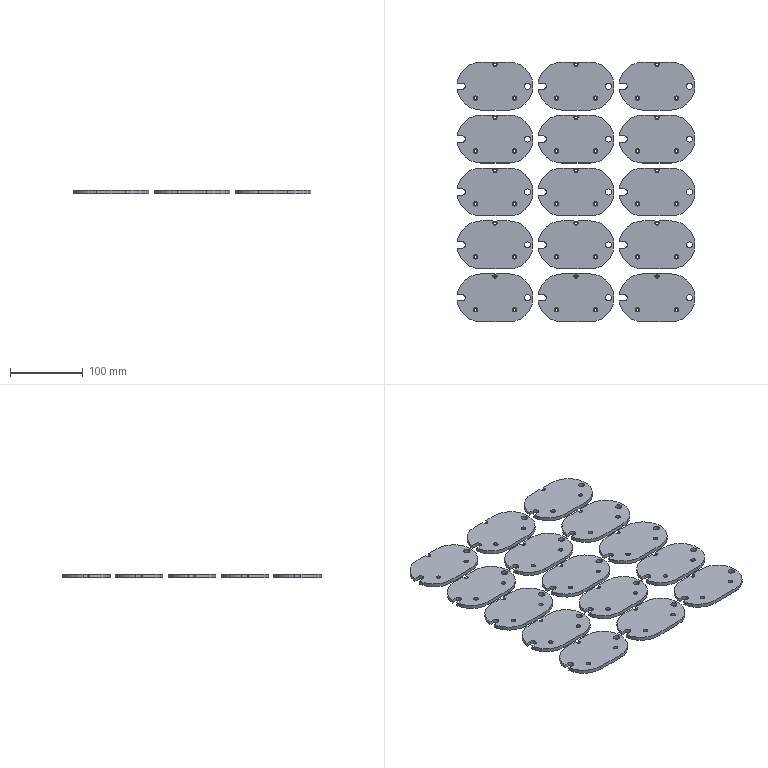NC program | NX | posted with a generic post | part box 328.125 x 358 x 5 mm
Lines 8101 to 9242 of 9242:
(PLANAR_MILL , TOOL : D6A45)
N16188 T14 M6
N16190 G54
N16192 G17 G0 G90 X15.634 Y-140.284 S9500 M3
N16194 G43 Z30. H14
N16196 Z0.
N16198 G94 G1 Z-1. F1250.
N16200 G3 X16.5 Y-140.784 R1.
N16202 X18.6 Y-138.684 R2.1
N16204 X16.5 Y-140.784 R-2.1
N16206 X17.366 Y-140.284 R1.
N16208 G1 Z0.
N16210 G0 Z30.
N16212 X34.4 Y-110.971
N16214 Z0.
N16216 G1 Z-1.
N16218 G3 X33.9 Y-111.837 R1.
N16220 G1 Y-131.337
N16222 G2 X4.366 Y-164.955 R33.9
N16224 X3.35 Y-164.063 R0.9
N16226 G1 Y-156.837
N16228 G3 X0. Y-153.487 R3.35
N16230 X-3.35 Y-156.837 R3.35
N16232 G1 Y-164.063
N16234 G2 X-4.366 Y-164.955 R0.9
N16236 X-33.9 Y-131.337 R33.9
N16238 G1 Y-114.837
N16240 G2 X-33. Y-113.937 R0.9
N16242 G1 X-30.
N16244 G3 X-27.9 Y-111.837 R2.1
N16246 X-30. Y-109.737 R2.1
N16248 G1 X-33.
N16250 G2 X-33.9 Y-108.837 R0.9
N16252 G1 Y-92.337
N16254 G2 X0. Y-58.437 R33.9
N16256 X33.9 Y-92.337 R33.9
N16258 G1 Y-111.837
N16260 G3 X34.4 Y-112.703 R1.
N16262 G1 Z0.
N16264 G0 Z30.
N16266 X15.634 Y-86.591
N16268 Z0.
N16270 G1 Z-1.
N16272 G3 X16.5 Y-87.091 R1.
N16274 X18.6 Y-84.991 R2.1
N16276 X16.5 Y-87.091 R-2.1
N16278 X17.366 Y-86.591 R1.
N16280 G1 Z0.
N16282 G0 Z30.
N16284 X-0.866 Y-69.687
N16286 Z0.
N16288 G1 Z-1.
N16290 G3 X0. Y-70.187 R1.
N16292 X3.35 Y-66.837 R3.35
N16294 X0. Y-70.187 R-3.35
N16296 X0.866 Y-69.687 R1.
N16298 G1 Z0.
N16300 G0 Z30.
N16302 X15.634 Y-28.584
N16304 Z0.
N16306 G1 Z-1.
N16308 G3 X16.5 Y-29.084 R1.
N16310 X18.6 Y-26.984 R2.1
N16312 X16.5 Y-29.084 R-2.1
N16314 X17.366 Y-28.584 R1.
N16316 G1 Z0.
N16318 G0 Z30.
N16320 X107.4 Y0.729
N16322 Z0.
N16324 G1 Z-1.
N16326 G3 X106.9 Y-0.137 R1.
N16328 G1 Y-19.637
N16330 G2 X77.366 Y-53.255 R33.9
N16332 X76.35 Y-52.363 R0.9
N16334 G1 Y-45.137
N16336 G3 X73. Y-41.787 R3.35
N16338 X69.65 Y-45.137 R3.35
N16340 G1 Y-52.363
N16342 G2 X68.634 Y-53.255 R0.9
N16344 X39.1 Y-19.637 R33.9
N16346 G1 Y-3.137
N16348 G2 X40. Y-2.237 R0.9
N16350 G1 X43.
N16352 G3 X45.1 Y-0.137 R2.1
N16354 X43. Y1.963 R2.1
N16356 G1 X40.
N16358 G2 X39.1 Y2.863 R0.9
N16360 G1 Y19.363
N16362 G2 X73. Y53.263 R33.9
N16364 X106.9 Y19.363 R33.9
N16366 G1 Y-0.137
N16368 G3 X107.4 Y-1.003 R1.
N16370 G1 Z0.
N16372 G0 Z30.
N16374 X91.1 Y-27.85
N16376 Z0.
N16378 G1 Z-1.
N16380 G3 X91.6 Y-26.984 R1.
N16382 X89.5 Y-24.884 R2.1
N16384 X91.6 Y-26.984 R-2.1
N16386 X91.1 Y-26.118 R1.
N16388 G1 Z0.
N16390 G0 Z30.
N16392 X72.134 Y-69.687
N16394 Z0.
N16396 G1 Z-1.
N16398 G3 X73. Y-70.187 R1.
N16400 X76.35 Y-66.837 R3.35
N16402 X73. Y-70.187 R-3.35
N16404 X73.866 Y-69.687 R1.
N16406 G1 Z0.
N16408 G0 Z30.
N16410 X88.634 Y-86.591
N16412 Z0.
N16414 G1 Z-1.
N16416 G3 X89.5 Y-87.091 R1.
N16418 X91.6 Y-84.991 R2.1
N16420 X89.5 Y-87.091 R-2.1
N16422 X90.366 Y-86.591 R1.
N16424 G1 Z0.
N16426 G0 Z30.
N16428 X107.4 Y-110.971
N16430 Z0.
N16432 G1 Z-1.
N16434 G3 X106.9 Y-111.837 R1.
N16436 G1 Y-131.337
N16438 G2 X77.366 Y-164.955 R33.9
N16440 X76.35 Y-164.063 R0.9
N16442 G1 Y-156.837
N16444 G3 X73. Y-153.487 R3.35
N16446 X69.65 Y-156.837 R3.35
N16448 G1 Y-164.063
N16450 G2 X68.634 Y-164.955 R0.9
N16452 X39.1 Y-131.337 R33.9
N16454 G1 Y-114.837
N16456 G2 X40. Y-113.937 R0.9
N16458 G1 X43.
N16460 G3 X45.1 Y-111.837 R2.1
N16462 X43. Y-109.737 R2.1
N16464 G1 X40.
N16466 G2 X39.1 Y-108.837 R0.9
N16468 G1 Y-92.337
N16470 G2 X73. Y-58.437 R33.9
N16472 X106.9 Y-92.337 R33.9
N16474 G1 Y-111.837
N16476 G3 X107.4 Y-112.703 R1.
N16478 G1 Z0.
N16480 G0 Z30.
N16482 X88.634 Y-140.284
N16484 Z0.
N16486 G1 Z-1.
N16488 G3 X89.5 Y-140.784 R1.
N16490 X91.6 Y-138.684 R2.1
N16492 X89.5 Y-140.784 R-2.1
N16494 X90.366 Y-140.284 R1.
N16496 G1 Z0.
N16498 G0 Z30.
N16500 X164.1 Y-139.55
N16502 Z0.
N16504 G1 Z-1.
N16506 G3 X164.6 Y-138.684 R1.
N16508 X162.5 Y-136.584 R2.1
N16510 X164.6 Y-138.684 R-2.1
N16512 X164.1 Y-137.818 R1.
N16514 G1 Z0.
N16516 G0 Z30.
N16518 X180.4 Y-110.971
N16520 Z0.
N16522 G1 Z-1.
N16524 G3 X179.9 Y-111.837 R1.
N16526 G1 Y-131.337
N16528 G2 X150.366 Y-164.955 R33.9
N16530 X149.35 Y-164.063 R0.9
N16532 G1 Y-156.837
N16534 G3 X146. Y-153.487 R3.35
N16536 X142.65 Y-156.837 R3.35
N16538 G1 Y-164.063
N16540 G2 X141.634 Y-164.955 R0.9
N16542 X112.1 Y-131.337 R33.9
N16544 G1 Y-114.837
N16546 G2 X113. Y-113.937 R0.9
N16548 G1 X116.
N16550 G3 X118.1 Y-111.837 R2.1
N16552 X116. Y-109.737 R2.1
N16554 G1 X113.
N16556 G2 X112.1 Y-108.837 R0.9
N16558 G1 Y-92.337
N16560 G2 X146. Y-58.437 R33.9
N16562 X179.9 Y-92.337 R33.9
N16564 G1 Y-111.837
N16566 G3 X180.4 Y-112.703 R1.
N16568 G1 Z0.
N16570 G0 Z30.
N16572 X164.1 Y-85.857
N16574 Z0.
N16576 G1 Z-1.
N16578 G3 X164.6 Y-84.991 R1.
N16580 X162.5 Y-82.891 R2.1
N16582 X164.6 Y-84.991 R-2.1
N16584 X164.1 Y-84.125 R1.
N16586 G1 Z0.
N16588 G0 Z30.
N16590 X148.85 Y-67.703
N16592 Z0.
N16594 G1 Z-1.
N16596 G3 X149.35 Y-66.837 R1.
N16598 X146. Y-63.487 R3.35
N16600 X149.35 Y-66.837 R-3.35
N16602 X148.85 Y-65.971 R1.
N16604 G1 Z0.
N16606 G0 Z30.
N16608 X164.1 Y-27.85
N16610 Z0.
N16612 G1 Z-1.
N16614 G3 X164.6 Y-26.984 R1.
N16616 X162.5 Y-24.884 R2.1
N16618 X164.6 Y-26.984 R-2.1
N16620 X164.1 Y-26.118 R1.
N16622 G1 Z0.
N16624 G0 Z30.
N16626 X180.4 Y0.729
N16628 Z0.
N16630 G1 Z-1.
N16632 G3 X179.9 Y-0.137 R1.
N16634 G1 Y-19.637
N16636 G2 X150.366 Y-53.255 R33.9
N16638 X149.35 Y-52.363 R0.9
N16640 G1 Y-45.137
N16642 G3 X146. Y-41.787 R3.35
N16644 X142.65 Y-45.137 R3.35
N16646 G1 Y-52.363
N16648 G2 X141.634 Y-53.255 R0.9
N16650 X112.1 Y-19.637 R33.9
N16652 G1 Y-3.137
N16654 G2 X113. Y-2.237 R0.9
N16656 G1 X116.
N16658 G3 X118.1 Y-0.137 R2.1
N16660 X116. Y1.963 R2.1
N16662 G1 X113.
N16664 G2 X112.1 Y2.863 R0.9
N16666 G1 Y19.363
N16668 G2 X146. Y53.263 R33.9
N16670 X179.9 Y19.363 R33.9
N16672 G1 Y-0.137
N16674 G3 X180.4 Y-1.003 R1.
N16676 G1 Z0.
N16678 G0 Z30.
N16680 X164.1 Y25.843
N16682 Z0.
N16684 G1 Z-1.
N16686 G3 X164.6 Y26.709 R1.
N16688 X162.5 Y28.809 R2.1
N16690 X164.6 Y26.709 R-2.1
N16692 X164.1 Y27.575 R1.
N16694 G1 Z0.
N16696 G0 Z30.
N16698 X148.85 Y43.997
N16700 Z0.
N16702 G1 Z-1.
N16704 G3 X149.35 Y44.863 R1.
N16706 X146. Y48.213 R3.35
N16708 X149.35 Y44.863 R-3.35
N16710 X148.85 Y45.729 R1.
N16712 G1 Z0.
N16714 G0 Z30.
N16716 X164.1 Y83.85
N16718 Z0.
N16720 G1 Z-1.
N16722 G3 X164.6 Y84.716 R1.
N16724 X162.5 Y86.816 R2.1
N16726 X164.6 Y84.716 R-2.1
N16728 X164.1 Y85.582 R1.
N16730 G1 Z0.
N16732 G0 Z30.
N16734 X180.4 Y112.429
N16736 Z0.
N16738 G1 Z-1.
N16740 G3 X179.9 Y111.563 R1.
N16742 G1 Y92.063
N16744 G2 X150.366 Y58.445 R33.9
N16746 X149.35 Y59.337 R0.9
N16748 G1 Y66.563
N16750 G3 X146. Y69.913 R3.35
N16752 X142.65 Y66.563 R3.35
N16754 G1 Y59.337
N16756 G2 X141.634 Y58.445 R0.9
N16758 X112.1 Y92.063 R33.9
N16760 G1 Y108.563
N16762 G2 X113. Y109.463 R0.9
N16764 G1 X116.
N16766 G3 X118.1 Y111.563 R2.1
N16768 X116. Y113.663 R2.1
N16770 G1 X113.
N16772 G2 X112.1 Y114.563 R0.9
N16774 G1 Y131.063
N16776 G2 X146. Y164.963 R33.9
N16778 X179.9 Y131.063 R33.9
N16780 G1 Y111.563
N16782 G3 X180.4 Y110.697 R1.
N16784 G1 Z0.
N16786 G0 Z30.
N16788 X164.1 Y137.543
N16790 Z0.
N16792 G1 Z-1.
N16794 G3 X164.6 Y138.409 R1.
N16796 X162.5 Y140.509 R2.1
N16798 X164.6 Y138.409 R-2.1
N16800 X164.1 Y139.275 R1.
N16802 G1 Z0.
N16804 G0 Z30.
N16806 X146.866 Y159.413
N16808 Z0.
N16810 G1 Z-1.
N16812 G3 X146. Y159.913 R1.
N16814 X142.65 Y156.563 R3.35
N16816 X146. Y159.913 R-3.35
N16818 X145.134 Y159.413 R1.
N16820 G1 Z0.
N16822 G0 Z30.
N16824 X90.366 Y140.009
N16826 Z0.
N16828 G1 Z-1.
N16830 G3 X89.5 Y140.509 R1.
N16832 X87.4 Y138.409 R2.1
N16834 X89.5 Y140.509 R-2.1
N16836 X88.634 Y140.009 R1.
N16838 G1 Z0.
N16840 G0 Z30.
N16842 X73.866 Y159.413
N16844 Z0.
N16846 G1 Z-1.
N16848 G3 X73. Y159.913 R1.
N16850 X69.65 Y156.563 R3.35
N16852 X73. Y159.913 R-3.35
N16854 X72.134 Y159.413 R1.
N16856 G1 Z0.
N16858 G0 Z30.
N16860 X107.4 Y112.429
N16862 Z0.
N16864 G1 Z-1.
N16866 G3 X106.9 Y111.563 R1.
N16868 G1 Y92.063
N16870 G2 X77.366 Y58.445 R33.9
N16872 X76.35 Y59.337 R0.9
N16874 G1 Y66.563
N16876 G3 X73. Y69.913 R3.35
N16878 X69.65 Y66.563 R3.35
N16880 G1 Y59.337
N16882 G2 X68.634 Y58.445 R0.9
N16884 X39.1 Y92.063 R33.9
N16886 G1 Y108.563
N16888 G2 X40. Y109.463 R0.9
N16890 G1 X43.
N16892 G3 X45.1 Y111.563 R2.1
N16894 X43. Y113.663 R2.1
N16896 G1 X40.
N16898 G2 X39.1 Y114.563 R0.9
N16900 G1 Y131.063
N16902 G2 X73. Y164.963 R33.9
N16904 X106.9 Y131.063 R33.9
N16906 G1 Y111.563
N16908 G3 X107.4 Y110.697 R1.
N16910 G1 Z0.
N16912 G0 Z30.
N16914 X90.366 Y86.316
N16916 Z0.
N16918 G1 Z-1.
N16920 G3 X89.5 Y86.816 R1.
N16922 X87.4 Y84.716 R2.1
N16924 X89.5 Y86.816 R-2.1
N16926 X88.634 Y86.316 R1.
N16928 G1 Z0.
N16930 G0 Z30.
N16932 X91.1 Y25.843
N16934 Z0.
N16936 G1 Z-1.
N16938 G3 X91.6 Y26.709 R1.
N16940 X89.5 Y28.809 R2.1
N16942 X91.6 Y26.709 R-2.1
N16944 X91.1 Y27.575 R1.
N16946 G1 Z0.
N16948 G0 Z30.
N16950 X75.85 Y43.997
N16952 Z0.
N16954 G1 Z-1.
N16956 G3 X76.35 Y44.863 R1.
N16958 X73. Y48.213 R3.35
N16960 X76.35 Y44.863 R-3.35
N16962 X75.85 Y45.729 R1.
N16964 G1 Z0.
N16966 G0 Z30.
N16968 X17.366 Y28.309
N16970 Z0.
N16972 G1 Z-1.
N16974 G3 X16.5 Y28.809 R1.
N16976 X14.4 Y26.709 R2.1
N16978 X16.5 Y28.809 R-2.1
N16980 X15.634 Y28.309 R1.
N16982 G1 Z0.
N16984 G0 Z30.
N16986 X34.4 Y0.729
N16988 Z0.
N16990 G1 Z-1.
N16992 G3 X33.9 Y-0.137 R1.
N16994 G1 Y-19.637
N16996 G2 X4.366 Y-53.255 R33.9
N16998 X3.35 Y-52.363 R0.9
N17000 G1 Y-45.137
N17002 G3 X0. Y-41.787 R3.35
N17004 X-3.35 Y-45.137 R3.35
N17006 G1 Y-52.363
N17008 G2 X-4.366 Y-53.255 R0.9
N17010 X-33.9 Y-19.637 R33.9
N17012 G1 Y-3.137
N17014 G2 X-33. Y-2.237 R0.9
N17016 G1 X-30.
N17018 G3 X-27.9 Y-0.137 R2.1
N17020 X-30. Y1.963 R2.1
N17022 G1 X-33.
N17024 G2 X-33.9 Y2.863 R0.9
N17026 G1 Y19.363
N17028 G2 X0. Y53.263 R33.9
N17030 X33.9 Y19.363 R33.9
N17032 G1 Y-0.137
N17034 G3 X34.4 Y-1.003 R1.
N17036 G1 Z0.
N17038 G0 Z30.
N17040 X0.866 Y47.713
N17042 Z0.
N17044 G1 Z-1.
N17046 G3 X0. Y48.213 R1.
N17048 X-3.35 Y44.863 R3.35
N17050 X0. Y48.213 R-3.35
N17052 X-0.866 Y47.713 R1.
N17054 G1 Z0.
N17056 G0 Z30.
N17058 X17.366 Y86.316
N17060 Z0.
N17062 G1 Z-1.
N17064 G3 X16.5 Y86.816 R1.
N17066 X14.4 Y84.716 R2.1
N17068 X16.5 Y86.816 R-2.1
N17070 X15.634 Y86.316 R1.
N17072 G1 Z0.
N17074 G0 Z30.
N17076 X34.4 Y112.429
N17078 Z0.
N17080 G1 Z-1.
N17082 G3 X33.9 Y111.563 R1.
N17084 G1 Y92.063
N17086 G2 X4.366 Y58.445 R33.9
N17088 X3.35 Y59.337 R0.9
N17090 G1 Y66.563
N17092 G3 X0. Y69.913 R3.35
N17094 X-3.35 Y66.563 R3.35
N17096 G1 Y59.337
N17098 G2 X-4.366 Y58.445 R0.9
N17100 X-33.9 Y92.063 R33.9
N17102 G1 Y108.563
N17104 G2 X-33. Y109.463 R0.9
N17106 G1 X-30.
N17108 G3 X-27.9 Y111.563 R2.1
N17110 X-30. Y113.663 R2.1
N17112 G1 X-33.
N17114 G2 X-33.9 Y114.563 R0.9
N17116 G1 Y131.063
N17118 G2 X0. Y164.963 R33.9
N17120 X33.9 Y131.063 R33.9
N17122 G1 Y111.563
N17124 G3 X34.4 Y110.697 R1.
N17126 G1 Z0.
N17128 G0 Z30.
N17130 X17.366 Y140.009
N17132 Z0.
N17134 G1 Z-1.
N17136 G3 X16.5 Y140.509 R1.
N17138 X14.4 Y138.409 R2.1
N17140 X16.5 Y140.509 R-2.1
N17142 X15.634 Y140.009 R1.
N17144 G1 Z0.
N17146 G0 Z30.
N17148 X0.866 Y159.413
N17150 Z0.
N17152 G1 Z-1.
N17154 G3 X0. Y159.913 R1.
N17156 X-3.35 Y156.563 R3.35
N17158 X0. Y159.913 R-3.35
N17160 X-0.866 Y159.413 R1.
N17162 G1 Z0.
N17164 G0 Z30.
N17166 X-55.634 Y140.009
N17168 Z0.
N17170 G1 Z-1.
N17172 G3 X-56.5 Y140.509 R1.
N17174 X-58.6 Y138.409 R2.1
N17176 X-56.5 Y140.509 R-2.1
N17178 X-57.366 Y140.009 R1.
N17180 G1 Z0.
N17182 G0 Z30.
N17184 X-72.134 Y159.413
N17186 Z0.
N17188 G1 Z-1.
N17190 G3 X-73. Y159.913 R1.
N17192 X-76.35 Y156.563 R3.35
N17194 X-73. Y159.913 R-3.35
N17196 X-73.866 Y159.413 R1.
N17198 G1 Z0.
N17200 G0 Z30.
N17202 X-38.6 Y112.429
N17204 Z0.
N17206 G1 Z-1.
N17208 G3 X-39.1 Y111.563 R1.
N17210 G1 Y92.063
N17212 G2 X-68.634 Y58.445 R33.9
N17214 X-69.65 Y59.337 R0.9
N17216 G1 Y66.563
N17218 G3 X-73. Y69.913 R3.35
N17220 X-76.35 Y66.563 R3.35
N17222 G1 Y59.337
N17224 G2 X-77.366 Y58.445 R0.9
N17226 X-106.9 Y92.063 R33.9
N17228 G1 Y108.563
N17230 G2 X-106. Y109.463 R0.9
N17232 G1 X-103.
N17234 G3 X-100.9 Y111.563 R2.1
N17236 X-103. Y113.663 R2.1
N17238 G1 X-106.
N17240 G2 X-106.9 Y114.563 R0.9
N17242 G1 Y131.063
N17244 G2 X-73. Y164.963 R33.9
N17246 X-39.1 Y131.063 R33.9
N17248 G1 Y111.563
N17250 G3 X-38.6 Y110.697 R1.
N17252 G1 Z0.
N17254 G0 Z30.
N17256 X-55.634 Y86.316
N17258 Z0.
N17260 G1 Z-1.
N17262 G3 X-56.5 Y86.816 R1.
N17264 X-58.6 Y84.716 R2.1
N17266 X-56.5 Y86.816 R-2.1
N17268 X-57.366 Y86.316 R1.
N17270 G1 Z0.
N17272 G0 Z30.
N17274 X-75.85 Y45.729
N17276 Z0.
N17278 G1 Z-1.
N17280 G3 X-76.35 Y44.863 R1.
N17282 X-73. Y41.513 R3.35
N17284 X-76.35 Y44.863 R-3.35
N17286 X-75.85 Y43.997 R1.
N17288 G1 Z0.
N17290 G0 Z30.
N17292 X-58.1 Y27.575
N17294 Z0.
N17296 G1 Z-1.
N17298 G3 X-58.6 Y26.709 R1.
N17300 X-56.5 Y24.609 R2.1
N17302 X-58.6 Y26.709 R-2.1
N17304 X-58.1 Y25.843 R1.
N17306 G1 Z0.
N17308 G0 Z30.
N17310 X-38.6 Y0.729
N17312 Z0.
N17314 G1 Z-1.
N17316 G3 X-39.1 Y-0.137 R1.
N17318 G1 Y-19.637
N17320 G2 X-68.634 Y-53.255 R33.9
N17322 X-69.65 Y-52.363 R0.9
N17324 G1 Y-45.137
N17326 G3 X-73. Y-41.787 R3.35
N17328 X-76.35 Y-45.137 R3.35
N17330 G1 Y-52.363
N17332 G2 X-77.366 Y-53.255 R0.9
N17334 X-106.9 Y-19.637 R33.9
N17336 G1 Y-3.137
N17338 G2 X-106. Y-2.237 R0.9
N17340 G1 X-103.
N17342 G3 X-100.9 Y-0.137 R2.1
N17344 X-103. Y1.963 R2.1
N17346 G1 X-106.
N17348 G2 X-106.9 Y2.863 R0.9
N17350 G1 Y19.363
N17352 G2 X-73. Y53.263 R33.9
N17354 X-39.1 Y19.363 R33.9
N17356 G1 Y-0.137
N17358 G3 X-38.6 Y-1.003 R1.
N17360 G1 Z0.
N17362 G0 Z30.
N17364 X-58.1 Y-26.118
N17366 Z0.
N17368 G1 Z-1.
N17370 G3 X-58.6 Y-26.984 R1.
N17372 X-56.5 Y-29.084 R2.1
N17374 X-58.6 Y-26.984 R-2.1
N17376 X-58.1 Y-27.85 R1.
N17378 G1 Z0.
N17380 G0 Z30.
N17382 X-73.866 Y-69.687
N17384 Z0.
N17386 G1 Z-1.
N17388 G3 X-73. Y-70.187 R1.
N17390 X-69.65 Y-66.837 R3.35
N17392 X-73. Y-70.187 R-3.35
N17394 X-72.134 Y-69.687 R1.
N17396 G1 Z0.
N17398 G0 Z30.
N17400 X-57.366 Y-86.591
N17402 Z0.
N17404 G1 Z-1.
N17406 G3 X-56.5 Y-87.091 R1.
N17408 X-54.4 Y-84.991 R2.1
N17410 X-56.5 Y-87.091 R-2.1
N17412 X-55.634 Y-86.591 R1.
N17414 G1 Z0.
N17416 G0 Z30.
N17418 X-38.6 Y-110.971
N17420 Z0.
N17422 G1 Z-1.
N17424 G3 X-39.1 Y-111.837 R1.
N17426 G1 Y-131.337
N17428 G2 X-68.634 Y-164.955 R33.9
N17430 X-69.65 Y-164.063 R0.9
N17432 G1 Y-156.837
N17434 G3 X-73. Y-153.487 R3.35
N17436 X-76.35 Y-156.837 R3.35
N17438 G1 Y-164.063
N17440 G2 X-77.366 Y-164.955 R0.9
N17442 X-106.9 Y-131.337 R33.9
N17444 G1 Y-114.837
N17446 G2 X-106. Y-113.937 R0.9
N17448 G1 X-103.
N17450 G3 X-100.9 Y-111.837 R2.1
N17452 X-103. Y-109.737 R2.1
N17454 G1 X-106.
N17456 G2 X-106.9 Y-108.837 R0.9
N17458 G1 Y-92.337
N17460 G2 X-73. Y-58.437 R33.9
N17462 X-39.1 Y-92.337 R33.9
N17464 G1 Y-111.837
N17466 G3 X-38.6 Y-112.703 R1.
N17468 G1 Z0.
N17470 G0 Z30.
N17472 X-57.366 Y-140.284
N17474 Z0.
N17476 G1 Z-1.
N17478 G3 X-56.5 Y-140.784 R1.
N17480 X-54.4 Y-138.684 R2.1
N17482 X-56.5 Y-140.784 R-2.1
N17484 X-55.634 Y-140.284 R1.
N17486 G1 Z0.
N17488 G0 Z30.
N17490 X-130.366
N17492 Z0.
N17494 G1 Z-1.
N17496 G3 X-129.5 Y-140.784 R1.
N17498 X-127.4 Y-138.684 R2.1
N17500 X-129.5 Y-140.784 R-2.1
N17502 X-128.634 Y-140.284 R1.
N17504 G1 Z0.
N17506 G0 Z30.
N17508 X-111.6 Y-110.971
N17510 Z0.
N17512 G1 Z-1.
N17514 G3 X-112.1 Y-111.837 R1.
N17516 G1 Y-131.337
N17518 G2 X-141.634 Y-164.955 R33.9
N17520 X-142.65 Y-164.063 R0.9
N17522 G1 Y-156.837
N17524 G3 X-146. Y-153.487 R3.35
N17526 X-149.35 Y-156.837 R3.35
N17528 G1 Y-164.063
N17530 G2 X-150.366 Y-164.955 R0.9
N17532 X-179.9 Y-131.337 R33.9
N17534 G1 Y-114.837
N17536 G2 X-179. Y-113.937 R0.9
N17538 G1 X-176.
N17540 G3 X-173.9 Y-111.837 R2.1
N17542 X-176. Y-109.737 R2.1
N17544 G1 X-179.
N17546 G2 X-179.9 Y-108.837 R0.9
N17548 G1 Y-92.337
N17550 G2 X-146. Y-58.437 R33.9
N17552 X-112.1 Y-92.337 R33.9
N17554 G1 Y-111.837
N17556 G3 X-111.6 Y-112.703 R1.
N17558 G1 Z0.
N17560 G0 Z30.
N17562 X-131.1 Y-84.125
N17564 Z0.
N17566 G1 Z-1.
N17568 G3 X-131.6 Y-84.991 R1.
N17570 X-129.5 Y-87.091 R2.1
N17572 X-131.6 Y-84.991 R-2.1
N17574 X-131.1 Y-85.857 R1.
N17576 G1 Z0.
N17578 G0 Z30.
N17580 X-148.85 Y-65.971
N17582 Z0.
N17584 G1 Z-1.
N17586 G3 X-149.35 Y-66.837 R1.
N17588 X-146. Y-70.187 R3.35
N17590 X-149.35 Y-66.837 R-3.35
N17592 X-148.85 Y-67.703 R1.
N17594 G1 Z0.
N17596 G0 Z30.
N17598 X-131.1 Y-26.118
N17600 Z0.
N17602 G1 Z-1.
N17604 G3 X-131.6 Y-26.984 R1.
N17606 X-129.5 Y-29.084 R2.1
N17608 X-131.6 Y-26.984 R-2.1
N17610 X-131.1 Y-27.85 R1.
N17612 G1 Z0.
N17614 G0 Z30.
N17616 X-111.6 Y0.729
N17618 Z0.
N17620 G1 Z-1.
N17622 G3 X-112.1 Y-0.137 R1.
N17624 G1 Y-19.637
N17626 G2 X-141.634 Y-53.255 R33.9
N17628 X-142.65 Y-52.363 R0.9
N17630 G1 Y-45.137
N17632 G3 X-146. Y-41.787 R3.35
N17634 X-149.35 Y-45.137 R3.35
N17636 G1 Y-52.363
N17638 G2 X-150.366 Y-53.255 R0.9
N17640 X-179.9 Y-19.637 R33.9
N17642 G1 Y-3.137
N17644 G2 X-179. Y-2.237 R0.9
N17646 G1 X-176.
N17648 G3 X-173.9 Y-0.137 R2.1
N17650 X-176. Y1.963 R2.1
N17652 G1 X-179.
N17654 G2 X-179.9 Y2.863 R0.9
N17656 G1 Y19.363
N17658 G2 X-146. Y53.263 R33.9
N17660 X-112.1 Y19.363 R33.9
N17662 G1 Y-0.137
N17664 G3 X-111.6 Y-1.003 R1.
N17666 G1 Z0.
N17668 G0 Z30.
N17670 X-131.1 Y27.575
N17672 Z0.
N17674 G1 Z-1.
N17676 G3 X-131.6 Y26.709 R1.
N17678 X-129.5 Y24.609 R2.1
N17680 X-131.6 Y26.709 R-2.1
N17682 X-131.1 Y25.843 R1.
N17684 G1 Z0.
N17686 G0 Z30.
N17688 X-148.85 Y45.729
N17690 Z0.
N17692 G1 Z-1.
N17694 G3 X-149.35 Y44.863 R1.
N17696 X-146. Y41.513 R3.35
N17698 X-149.35 Y44.863 R-3.35
N17700 X-148.85 Y43.997 R1.
N17702 G1 Z0.
N17704 G0 Z30.
N17706 X-131.1 Y85.582
N17708 Z0.
N17710 G1 Z-1.
N17712 G3 X-131.6 Y84.716 R1.
N17714 X-129.5 Y82.616 R2.1
N17716 X-131.6 Y84.716 R-2.1
N17718 X-131.1 Y83.85 R1.
N17720 G1 Z0.
N17722 G0 Z30.
N17724 X-111.6 Y112.429
N17726 Z0.
N17728 G1 Z-1.
N17730 G3 X-112.1 Y111.563 R1.
N17732 G1 Y92.063
N17734 G2 X-141.634 Y58.445 R33.9
N17736 X-142.65 Y59.337 R0.9
N17738 G1 Y66.563
N17740 G3 X-146. Y69.913 R3.35
N17742 X-149.35 Y66.563 R3.35
N17744 G1 Y59.337
N17746 G2 X-150.366 Y58.445 R0.9
N17748 X-179.9 Y92.063 R33.9
N17750 G1 Y108.563
N17752 G2 X-179. Y109.463 R0.9
N17754 G1 X-176.
N17756 G3 X-173.9 Y111.563 R2.1
N17758 X-176. Y113.663 R2.1
N17760 G1 X-179.
N17762 G2 X-179.9 Y114.563 R0.9
N17764 G1 Y131.063
N17766 G2 X-146. Y164.963 R33.9
N17768 X-112.1 Y131.063 R33.9
N17770 G1 Y111.563
N17772 G3 X-111.6 Y110.697 R1.
N17774 G1 Z0.
N17776 G0 Z30.
N17778 X-128.634 Y140.009
N17780 Z0.
N17782 G1 Z-1.
N17784 G3 X-129.5 Y140.509 R1.
N17786 X-131.6 Y138.409 R2.1
N17788 X-129.5 Y140.509 R-2.1
N17790 X-130.366 Y140.009 R1.
N17792 G1 Z0.
N17794 G0 Z30.
N17796 X-145.134 Y159.413
N17798 Z0.
N17800 G1 Z-1.
N17802 G3 X-146. Y159.913 R1.
N17804 X-149.35 Y156.563 R3.35
N17806 X-146. Y159.913 R-3.35
N17808 X-146.866 Y159.413 R1.
N17810 G1 Z0.
N17812 G0 Z30.
N17814 M5
(ZLEVEL_PROFILE_COPY , TOOL : D6)
N17816 T06 M6
N17818 G54
N17820 G17 G0 G90 X-72.289 Y58.68 S7500 M3
N17822 G43 Z30. H6
N17824 Z-3.85
N17826 G94 G1 Z-4.85 F1000.
N17828 X-72.05 Y58.818
N17830 G3 X-71.75 Y59.337 R0.6
N17832 G1 Y66.563
N17834 G3 X-73. Y67.813 R1.25
N17836 X-74.25 Y66.563 R1.25
N17838 G1 Y59.337
N17840 G2 X-77.648 Y56.364 R3.
N17842 X-109. Y92.063 R36.
N17844 G1 Y131.063
N17846 G2 X-73. Y167.063 R36.
N17848 X-37. Y131.063 R36.
N17850 G1 Y92.063
N17852 G2 X-68.364 Y56.362 R36.
N17854 X-71.75 Y59.337 R3.
N17856 G3 X-72.05 Y59.857 R0.6
N17858 G1 X-72.35 Y60.03
N17860 Z-4.25
N17862 G0 Z30.
N17864 X182.594 Y-91.648
N17866 Z-3.85
N17868 G1 Z-4.85
N17870 X182.3 Y-91.818
N17872 G3 X182. Y-92.337 R0.6
N17874 G1 Y-131.337
N17876 G2 X150.636 Y-167.038 R36.
N17878 X147.25 Y-164.063 R3.
N17880 G1 Y-156.837
N17882 G3 X146. Y-155.587 R1.25
N17884 X144.75 Y-156.837 R1.25
N17886 G1 Y-164.063
N17888 G2 X141.346 Y-167.035 R3.
N17890 X110. Y-131.337 R36.
N17892 G1 Y-92.337
N17894 G2 X146. Y-56.337 R36.
N17896 X182. Y-92.337 R36.
N17898 G3 X182.3 Y-92.857 R0.6
N17900 G1 X182.6 Y-93.03
N17902 Z-4.25
N17904 G0 Z30.
N17906 X182.594 Y20.052
N17908 Z-3.85
N17910 G1 Z-4.85
N17912 X182.3 Y19.882
N17914 G3 X182. Y19.363 R0.6
N17916 G1 Y-19.637
N17918 G2 X150.636 Y-55.338 R36.
N17920 X147.25 Y-52.333 R3.
N17922 G1 Y-45.137
N17924 G3 X146. Y-43.887 R1.25
N17926 X144.75 Y-45.137 R1.25
N17928 G1 Y-52.363
N17930 G2 X141.346 Y-55.335 R3.
N17932 X110. Y-19.637 R36.
N17934 G1 Y19.363
N17936 G2 X146. Y55.363 R36.
N17938 X182. Y19.363 R36.
N17940 G3 X182.3 Y18.843 R0.6
N17942 G1 X182.6 Y18.67
N17944 Z-4.25
N17946 G0 Z30.
N17948 X0.711 Y-164.72
N17950 Z-3.85
N17952 G1 Z-4.85
N17954 X0.95 Y-164.582
N17956 G3 X1.25 Y-164.063 R0.6
N17958 G1 Y-156.837
N17960 G3 X0. Y-155.587 R1.25
N17962 X-1.25 Y-156.837 R1.25
N17964 G1 Y-164.063
N17966 G2 X-4.665 Y-167.034 R3.
N17968 X-36. Y-131.337 R36.
N17970 G1 Y-92.337
N17972 G2 X0. Y-56.337 R36.
N17974 X36. Y-92.337 R36.
N17976 G1 Y-131.337
N17978 G2 X4.636 Y-167.038 R36.
N17980 X1.25 Y-164.063 R3.
N17982 G3 X0.95 Y-163.543 R0.6
N17984 G1 X0.65 Y-163.37
N17986 Z-4.25
N17988 G0 Z30.
N17990 X-72.289 Y-164.72
N17992 Z-3.85
N17994 G1 Z-4.85
N17996 X-72.05 Y-164.582
N17998 G3 X-71.75 Y-164.063 R0.6
N18000 G1 Y-156.837
N18002 G3 X-73. Y-155.587 R1.25
N18004 X-74.25 Y-156.837 R1.25
N18006 G1 Y-164.063
N18008 G2 X-77.648 Y-167.036 R3.
N18010 X-109. Y-131.337 R36.
N18012 G1 Y-92.337
N18014 G2 X-73. Y-56.337 R36.
N18016 X-37. Y-92.337 R36.
N18018 G1 Y-131.337
N18020 G2 X-68.364 Y-167.038 R36.
N18022 X-71.75 Y-164.063 R3.
N18024 G3 X-72.05 Y-163.543 R0.6
N18026 G1 X-72.35 Y-163.37
N18028 Z-4.25
N18030 G0 Z30.
N18032 X182.594 Y131.752
N18034 Z-3.85
N18036 G1 Z-4.85
N18038 X182.3 Y131.582
N18040 G3 X182. Y131.063 R0.6
N18042 G1 Y92.063
N18044 G2 X150.636 Y56.362 R36.
N18046 X147.25 Y59.359 R3.
N18048 G1 Y66.563
N18050 G3 X146. Y67.813 R1.25
N18052 X144.75 Y66.563 R1.25
N18054 G1 Y59.337
N18056 G2 X141.346 Y56.365 R3.
N18058 X110. Y92.063 R36.
N18060 G1 Y131.063
N18062 G2 X146. Y167.063 R36.
N18064 X182. Y131.063 R36.
N18066 G3 X182.3 Y130.543 R0.6
N18068 G1 X182.6 Y130.37
N18070 Z-4.25
N18072 G0 Z30.
N18074 X-182.594 Y-132.026
N18076 Z-3.85
N18078 G1 Z-4.85
N18080 X-182.3 Y-131.857
N18082 G3 X-182. Y-131.337 R0.6
N18084 G1 Y-92.337
N18086 G2 X-146. Y-56.337 R36.
N18088 X-110. Y-92.337 R36.
N18090 G1 Y-131.337
N18092 G2 X-141.364 Y-167.038 R36.
N18094 X-144.75 Y-164.063 R3.
N18096 G1 Y-156.837
N18098 G3 X-146. Y-155.587 R1.25
N18100 X-147.25 Y-156.837 R1.25
N18102 G1 Y-164.063
N18104 G2 X-150.585 Y-167.044 R3.
N18106 G1 X-150.682 Y-167.032
N18108 G2 X-182. Y-131.337 R36.
N18110 G3 X-182.3 Y-130.818 R0.6
N18112 G1 X-182.6 Y-130.645
N18114 Z-4.25
N18116 G0 Z30.
N18118 X-0.57 Y-44.825
N18120 Z-3.85
N18122 G1 Z-4.85
N18124 X-0.95 Y-44.618
N18126 G3 X-1.25 Y-45.137 R0.6
N18128 G1 Y-52.363
N18130 G2 X-4.602 Y-55.342 R3.
N18132 G1 X-4.694 Y-55.33
N18134 G2 X-36. Y-19.637 R36.
N18136 G1 Y19.363
N18138 G2 X0. Y55.363 R36.
N18140 X36. Y19.363 R36.
N18142 G1 Y-19.637
N18144 G2 X4.636 Y-55.338 R36.
N18146 X1.25 Y-52.333 R3.
N18148 G1 Y-45.137
N18150 G3 X0. Y-43.887 R1.25
N18152 X-1.25 Y-45.137 R1.25
N18154 X-0.95 Y-45.657 R0.6
N18156 G1 X-0.65 Y-45.83
N18158 Z-4.25
N18160 G0 Z30.
N18162 X73.711 Y-53.02
N18164 Z-3.85
N18166 G1 Z-4.85
N18168 X73.95 Y-52.882
N18170 G3 X74.25 Y-52.363 R0.6
N18172 G1 Y-45.137
N18174 G3 X73. Y-43.887 R1.25
N18176 X71.75 Y-45.137 R1.25
N18178 G1 Y-52.363
N18180 G2 X68.326 Y-55.333 R3.
N18182 X37. Y-19.637 R36.
N18184 G1 Y19.363
N18186 G2 X73. Y55.363 R36.
N18188 X109. Y19.363 R36.
N18190 G1 Y-19.637
N18192 G2 X77.636 Y-55.338 R36.
N18194 X74.25 Y-52.363 R3.
N18196 G3 X73.95 Y-51.843 R0.6
N18198 G1 X73.65 Y-51.67
N18200 Z-4.25
N18202 G0 Z30.
N18204 X-73.57 Y-44.825
N18206 Z-3.85
N18208 G1 Z-4.85
N18210 X-73.95 Y-44.618
N18212 G3 X-74.25 Y-45.137 R0.6
N18214 G1 Y-52.363
N18216 G2 X-77.648 Y-55.336 R3.
N18218 X-109. Y-19.637 R36.
N18220 G1 Y19.363
N18222 G2 X-73. Y55.363 R36.
N18224 X-37. Y19.363 R36.
N18226 G1 Y-19.637
N18228 G2 X-68.364 Y-55.338 R36.
N18230 X-71.75 Y-52.333 R3.
N18232 G1 Y-45.137
N18234 G3 X-73. Y-43.887 R1.25
N18236 X-74.25 Y-45.137 R1.25
N18238 X-73.95 Y-45.657 R0.6
N18240 G1 X-73.65 Y-45.83
N18242 Z-4.25
N18244 G0 Z30.
N18246 X73.711 Y58.68
N18248 Z-3.85
N18250 G1 Z-4.85
N18252 X73.95 Y58.818
N18254 G3 X74.25 Y59.337 R0.6
N18256 G1 Y66.563
N18258 G3 X73. Y67.813 R1.25
N18260 X71.75 Y66.563 R1.25
N18262 G1 Y59.337
N18264 G2 X68.345 Y56.365 R3.
N18266 X37. Y92.063 R36.
N18268 G1 Y131.063
N18270 G2 X73. Y167.063 R36.
N18272 X109. Y131.063 R36.
N18274 G1 Y92.063
N18276 G2 X77.636 Y56.362 R36.
N18278 X74.25 Y59.337 R3.
N18280 G3 X73.95 Y59.857 R0.6
N18282 G1 X73.65 Y60.03
N18284 Z-4.25
N18286 G0 Z30.
N18288 X0.711 Y58.68
N18290 Z-3.85
N18292 G1 Z-4.85
N18294 X0.95 Y58.818
N18296 G3 X1.25 Y59.337 R0.6
N18298 G1 Y66.563
N18300 G3 X0. Y67.813 R1.25
N18302 X-1.25 Y66.563 R1.25
N18304 G1 Y59.337
N18306 G2 X-4.665 Y56.366 R3.
N18308 X-36. Y92.063 R36.
N18310 G1 Y131.063
N18312 G2 X0. Y167.063 R36.
N18314 X36. Y131.063 R36.
N18316 G1 Y92.063
N18318 G2 X4.636 Y56.362 R36.
N18320 X1.25 Y59.337 R3.
N18322 G3 X0.95 Y59.857 R0.6
N18324 G1 X0.65 Y60.03
N18326 Z-4.25
N18328 G0 Z30.
N18330 X-182.594 Y91.374
N18332 Z-3.85
N18334 G1 Z-4.85
N18336 X-182.3 Y91.543
N18338 G3 X-182. Y92.063 R0.6
N18340 G1 Y131.063
N18342 G2 X-146. Y167.063 R36.
N18344 X-110. Y131.063 R36.
N18346 G1 Y92.063
N18348 G2 X-141.364 Y56.362 R36.
N18350 X-144.75 Y59.359 R3.
N18352 G1 Y66.563
N18354 G3 X-146. Y67.813 R1.25
N18356 X-147.25 Y66.563 R1.25
N18358 G1 Y59.337
N18360 G2 X-150.659 Y56.365 R3.
N18362 X-182. Y92.063 R36.
N18364 G3 X-182.3 Y92.582 R0.6
N18366 G1 X-182.6 Y92.755
N18368 Z-4.25
N18370 G0 Z30.
N18372 X73.711 Y-164.72
N18374 Z-3.85
N18376 G1 Z-4.85
N18378 X73.95 Y-164.582
N18380 G3 X74.25 Y-164.063 R0.6
N18382 G1 Y-156.837
N18384 G3 X73. Y-155.587 R1.25
N18386 X71.75 Y-156.837 R1.25
N18388 G1 Y-164.063
N18390 G2 X68.345 Y-167.035 R3.
N18392 X37. Y-131.337 R36.
N18394 G1 Y-92.337
N18396 G2 X73. Y-56.337 R36.
N18398 X109. Y-92.337 R36.
N18400 G1 Y-131.337
N18402 G2 X77.636 Y-167.038 R36.
N18404 X74.25 Y-164.063 R3.
N18406 G3 X73.95 Y-163.543 R0.6
N18408 G1 X73.65 Y-163.37
N18410 Z-4.25
N18412 G0 Z30.
N18414 X-182.594 Y-20.326
N18416 Z-3.85
N18418 G1 Z-4.85
N18420 X-182.3 Y-20.157
N18422 G3 X-182. Y-19.637 R0.6
N18424 G1 Y19.363
N18426 G2 X-146. Y55.363 R36.
N18428 X-110. Y19.363 R36.
N18430 G1 Y-19.637
N18432 G2 X-141.364 Y-55.338 R36.
N18434 X-144.75 Y-52.333 R3.
N18436 G1 Y-45.137
N18438 G3 X-146. Y-43.887 R1.25
N18440 X-147.25 Y-45.137 R1.25
N18442 G1 Y-52.363
N18444 G2 X-150.659 Y-55.335 R3.
N18446 X-182. Y-19.637 R36.
N18448 G3 X-182.3 Y-19.118 R0.6
N18450 G1 X-182.6 Y-18.945
N18452 Z-4.25
N18454 G0 Z30.
N18456 M5
N18458 M2